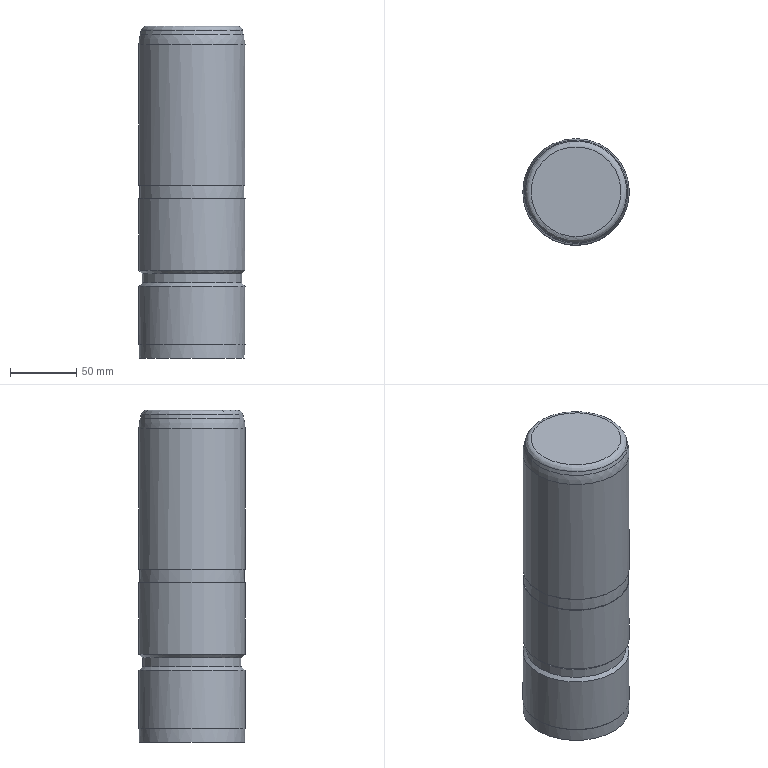Part | NX | features solid 2 | 1 solid | 16 faces | box 80 x 80 x 250 mm | volume 1244974 mm3 | cylinder 6 | plane 5 | cone 3 | torus 2 | commonest cylinder face diameters 80 x3 75 x1 79 x1 79.5 x1
STEP:
#1=CARTESIAN_POINT('',(1067.5,-565.,-201.5));
#2=VERTEX_POINT('',#1);
#3=CARTESIAN_POINT('',(1030.,-565.,-201.5));
#4=DIRECTION('',(0.,0.,-1.));
#5=DIRECTION('',(1.,0.,0.));
#6=AXIS2_PLACEMENT_3D('',#3,#4,#5);
#7=CIRCLE('',#6,37.5);
#8=EDGE_CURVE('',#2,#2,#7,.T.);
#9=ORIENTED_EDGE('',*,*,#8,.F.);
#10=EDGE_LOOP('',(#9));
#11=FACE_BOUND('',#10,.T.);
#12=CARTESIAN_POINT('',(990.,-565.,-199.));
#13=VERTEX_POINT('',#12);
#14=CARTESIAN_POINT('',(1030.,-565.,-199.));
#15=DIRECTION('',(0.,0.,1.));
#16=DIRECTION('',(-1.,0.,0.));
#17=AXIS2_PLACEMENT_3D('',#14,#15,#16);
#18=CIRCLE('',#17,40.);
#19=EDGE_CURVE('',#13,#13,#18,.T.);
#20=ORIENTED_EDGE('',*,*,#19,.F.);
#21=EDGE_LOOP('',(#20));
#22=FACE_BOUND('',#21,.T.);
#23=CARTESIAN_POINT('',(1030.,-565.,-201.5));
#24=DIRECTION('',(0.,0.,1.));
#25=DIRECTION('',(-1.,0.,0.));
#26=AXIS2_PLACEMENT_3D('',#23,#24,#25);
#27=CONICAL_SURFACE('',#26,37.5,0.7854);
#28=ADVANCED_FACE('',(#11,#22),#27,.T.);
#29=ORIENTED_EDGE('',*,*,#8,.T.);
#30=EDGE_LOOP('',(#29));
#31=FACE_BOUND('',#30,.T.);
#32=CARTESIAN_POINT('',(1067.5,-565.,-208.5));
#33=VERTEX_POINT('',#32);
#34=CARTESIAN_POINT('',(1030.,-565.,-208.5));
#35=DIRECTION('',(0.,0.,-1.));
#36=DIRECTION('',(1.,0.,0.));
#37=AXIS2_PLACEMENT_3D('',#34,#35,#36);
#38=CIRCLE('',#37,37.5);
#39=EDGE_CURVE('',#33,#33,#38,.T.);
#40=ORIENTED_EDGE('',*,*,#39,.F.);
#41=EDGE_LOOP('',(#40));
#42=FACE_BOUND('',#41,.T.);
#43=CARTESIAN_POINT('',(1030.,-565.,-208.5));
#44=DIRECTION('',(0.,0.,1.));
#45=DIRECTION('',(-1.,0.,0.));
#46=AXIS2_PLACEMENT_3D('',#43,#44,#45);
#47=CYLINDRICAL_SURFACE('',#46,37.5);
#48=ADVANCED_FACE('',(#31,#42),#47,.T.);
#49=CARTESIAN_POINT('',(990.5,-565.,-145.));
#50=VERTEX_POINT('',#49);
#51=CARTESIAN_POINT('',(1030.,-565.,-145.));
#52=DIRECTION('',(0.,0.,1.));
#53=DIRECTION('',(-1.,0.,0.));
#54=AXIS2_PLACEMENT_3D('',#51,#52,#53);
#55=CIRCLE('',#54,39.5);
#56=EDGE_CURVE('',#50,#50,#55,.T.);
#57=ORIENTED_EDGE('',*,*,#56,.F.);
#58=EDGE_LOOP('',(#57));
#59=FACE_BOUND('',#58,.T.);
#60=CARTESIAN_POINT('',(1070.,-565.,-145.));
#61=VERTEX_POINT('',#60);
#62=CARTESIAN_POINT('',(1030.,-565.,-145.));
#63=DIRECTION('',(0.,0.,-1.));
#64=DIRECTION('',(1.,0.,0.));
#65=AXIS2_PLACEMENT_3D('',#62,#63,#64);
#66=CIRCLE('',#65,40.);
#67=EDGE_CURVE('',#61,#61,#66,.T.);
#68=ORIENTED_EDGE('',*,*,#67,.F.);
#69=EDGE_LOOP('',(#68));
#70=FACE_BOUND('',#69,.T.);
#71=CARTESIAN_POINT('',(1030.,-565.,-145.));
#72=DIRECTION('',(0.,0.,1.));
#73=DIRECTION('',(-1.,0.,0.));
#74=AXIS2_PLACEMENT_3D('',#71,#72,#73);
#75=PLANE('',#74);
#76=ADVANCED_FACE('',(#59,#70),#75,.T.);
#77=ORIENTED_EDGE('',*,*,#67,.T.);
#78=EDGE_LOOP('',(#77));
#79=FACE_BOUND('',#78,.T.);
#80=ORIENTED_EDGE('',*,*,#19,.T.);
#81=EDGE_LOOP('',(#80));
#82=FACE_BOUND('',#81,.T.);
#83=CARTESIAN_POINT('',(1030.,-565.,-199.));
#84=DIRECTION('',(0.,0.,1.));
#85=DIRECTION('',(-1.,0.,0.));
#86=AXIS2_PLACEMENT_3D('',#83,#84,#85);
#87=CYLINDRICAL_SURFACE('',#86,40.);
#88=ADVANCED_FACE('',(#79,#82),#87,.T.);
#89=CARTESIAN_POINT('',(1069.5,-565.,-135.));
#90=VERTEX_POINT('',#89);
#91=CARTESIAN_POINT('',(1030.,-565.,-135.));
#92=DIRECTION('',(0.,0.,-1.));
#93=DIRECTION('',(1.,0.,0.));
#94=AXIS2_PLACEMENT_3D('',#91,#92,#93);
#95=CIRCLE('',#94,39.5);
#96=EDGE_CURVE('',#90,#90,#95,.T.);
#97=ORIENTED_EDGE('',*,*,#96,.F.);
#98=EDGE_LOOP('',(#97));
#99=FACE_BOUND('',#98,.T.);
#100=CARTESIAN_POINT('',(990.,-565.,-135.));
#101=VERTEX_POINT('',#100);
#102=CARTESIAN_POINT('',(1030.,-565.,-135.));
#103=DIRECTION('',(0.,0.,1.));
#104=DIRECTION('',(-1.,0.,0.));
#105=AXIS2_PLACEMENT_3D('',#102,#103,#104);
#106=CIRCLE('',#105,40.);
#107=EDGE_CURVE('',#101,#101,#106,.T.);
#108=ORIENTED_EDGE('',*,*,#107,.F.);
#109=EDGE_LOOP('',(#108));
#110=FACE_BOUND('',#109,.T.);
#111=CARTESIAN_POINT('',(1030.,-565.,-135.));
#112=DIRECTION('',(0.,0.,-1.));
#113=DIRECTION('',(1.,0.,0.));
#114=AXIS2_PLACEMENT_3D('',#111,#112,#113);
#115=PLANE('',#114);
#116=ADVANCED_FACE('',(#99,#110),#115,.T.);
#117=CARTESIAN_POINT('',(1070.,-565.,-28.95));
#118=VERTEX_POINT('',#117);
#119=CARTESIAN_POINT('',(1030.,-565.,-28.95));
#120=DIRECTION('',(0.,0.,-1.));
#121=DIRECTION('',(1.,0.,0.));
#122=AXIS2_PLACEMENT_3D('',#119,#120,#121);
#123=CIRCLE('',#122,40.);
#124=EDGE_CURVE('',#118,#118,#123,.T.);
#125=ORIENTED_EDGE('',*,*,#124,.T.);
#126=EDGE_LOOP('',(#125));
#127=FACE_BOUND('',#126,.T.);
#128=ORIENTED_EDGE('',*,*,#107,.T.);
#129=EDGE_LOOP('',(#128));
#130=FACE_BOUND('',#129,.T.);
#131=CARTESIAN_POINT('',(1030.,-565.,-135.));
#132=DIRECTION('',(0.,0.,1.));
#133=DIRECTION('',(-1.,0.,0.));
#134=AXIS2_PLACEMENT_3D('',#131,#132,#133);
#135=CYLINDRICAL_SURFACE('',#134,40.);
#136=ADVANCED_FACE('',(#127,#130),#135,.T.);
#137=ORIENTED_EDGE('',*,*,#96,.T.);
#138=EDGE_LOOP('',(#137));
#139=FACE_BOUND('',#138,.T.);
#140=ORIENTED_EDGE('',*,*,#56,.T.);
#141=EDGE_LOOP('',(#140));
#142=FACE_BOUND('',#141,.T.);
#143=CARTESIAN_POINT('',(1030.,-565.,-145.));
#144=DIRECTION('',(0.,0.,1.));
#145=DIRECTION('',(-1.,0.,0.));
#146=AXIS2_PLACEMENT_3D('',#143,#144,#145);
#147=CYLINDRICAL_SURFACE('',#146,39.5);
#148=ADVANCED_FACE('',(#139,#142),#147,.T.);
#149=CARTESIAN_POINT('',(996.132,-565.,-15.));
#150=VERTEX_POINT('',#149);
#151=CARTESIAN_POINT('',(1030.,-565.,-15.));
#152=DIRECTION('',(0.,0.,1.));
#153=DIRECTION('',(-1.,0.,0.));
#154=AXIS2_PLACEMENT_3D('',#151,#152,#153);
#155=CIRCLE('',#154,33.868);
#156=EDGE_CURVE('',#150,#150,#155,.T.);
#157=ORIENTED_EDGE('',*,*,#156,.T.);
#158=EDGE_LOOP('',(#157));
#159=FACE_BOUND('',#158,.T.);
#160=CARTESIAN_POINT('',(1030.,-565.,-15.));
#161=DIRECTION('',(0.,0.,1.));
#162=DIRECTION('',(-1.,0.,0.));
#163=AXIS2_PLACEMENT_3D('',#160,#161,#162);
#164=PLANE('',#163);
#165=ADVANCED_FACE('',(#159),#164,.T.);
#166=CARTESIAN_POINT('',(991.786,-565.,-18.335));
#167=VERTEX_POINT('',#166);
#168=CARTESIAN_POINT('',(1030.,-565.,-18.335));
#169=DIRECTION('',(0.,0.,1.));
#170=DIRECTION('',(-1.,0.,0.));
#171=AXIS2_PLACEMENT_3D('',#168,#169,#170);
#172=CIRCLE('',#171,38.214);
#173=EDGE_CURVE('',#167,#167,#172,.F.);
#174=ORIENTED_EDGE('',*,*,#173,.T.);
#175=EDGE_LOOP('',(#174));
#176=FACE_BOUND('',#175,.T.);
#177=CARTESIAN_POINT('',(991.022,-565.,-21.185));
#178=VERTEX_POINT('',#177);
#179=CARTESIAN_POINT('',(1030.,-565.,-21.185));
#180=DIRECTION('',(0.,0.,1.));
#181=DIRECTION('',(-1.,0.,0.));
#182=AXIS2_PLACEMENT_3D('',#179,#180,#181);
#183=CIRCLE('',#182,38.978);
#184=EDGE_CURVE('',#178,#178,#183,.T.);
#185=ORIENTED_EDGE('',*,*,#184,.T.);
#186=EDGE_LOOP('',(#185));
#187=FACE_BOUND('',#186,.T.);
#188=CARTESIAN_POINT('',(1030.,-565.,-15.));
#189=DIRECTION('',(0.,0.,-1.));
#190=DIRECTION('',(1.,0.,0.));
#191=AXIS2_PLACEMENT_3D('',#188,#189,#190);
#192=CONICAL_SURFACE('',#191,37.321,0.2618);
#193=ADVANCED_FACE('',(#176,#187),#192,.T.);
#194=CARTESIAN_POINT('',(1069.75,-565.,-255.));
#195=VERTEX_POINT('',#194);
#196=CARTESIAN_POINT('',(1030.,-565.,-255.));
#197=DIRECTION('',(0.,0.,-1.));
#198=DIRECTION('',(1.,0.,0.));
#199=AXIS2_PLACEMENT_3D('',#196,#197,#198);
#200=CIRCLE('',#199,39.75);
#201=EDGE_CURVE('',#195,#195,#200,.T.);
#202=ORIENTED_EDGE('',*,*,#201,.F.);
#203=EDGE_LOOP('',(#202));
#204=FACE_BOUND('',#203,.T.);
#205=CARTESIAN_POINT('',(990.,-565.,-255.));
#206=VERTEX_POINT('',#205);
#207=CARTESIAN_POINT('',(1030.,-565.,-255.));
#208=DIRECTION('',(0.,0.,1.));
#209=DIRECTION('',(-1.,0.,0.));
#210=AXIS2_PLACEMENT_3D('',#207,#208,#209);
#211=CIRCLE('',#210,40.);
#212=EDGE_CURVE('',#206,#206,#211,.T.);
#213=ORIENTED_EDGE('',*,*,#212,.F.);
#214=EDGE_LOOP('',(#213));
#215=FACE_BOUND('',#214,.T.);
#216=CARTESIAN_POINT('',(1030.,-565.,-255.));
#217=DIRECTION('',(0.,0.,-1.));
#218=DIRECTION('',(1.,0.,0.));
#219=AXIS2_PLACEMENT_3D('',#216,#217,#218);
#220=PLANE('',#219);
#221=ADVANCED_FACE('',(#204,#215),#220,.T.);
#222=CARTESIAN_POINT('',(990.,-565.,-211.));
#223=VERTEX_POINT('',#222);
#224=CARTESIAN_POINT('',(1030.,-565.,-211.));
#225=DIRECTION('',(0.,0.,1.));
#226=DIRECTION('',(-1.,0.,0.));
#227=AXIS2_PLACEMENT_3D('',#224,#225,#226);
#228=CIRCLE('',#227,40.);
#229=EDGE_CURVE('',#223,#223,#228,.T.);
#230=ORIENTED_EDGE('',*,*,#229,.F.);
#231=EDGE_LOOP('',(#230));
#232=FACE_BOUND('',#231,.T.);
#233=ORIENTED_EDGE('',*,*,#212,.T.);
#234=EDGE_LOOP('',(#233));
#235=FACE_BOUND('',#234,.T.);
#236=CARTESIAN_POINT('',(1030.,-565.,-255.));
#237=DIRECTION('',(0.,0.,1.));
#238=DIRECTION('',(-1.,0.,0.));
#239=AXIS2_PLACEMENT_3D('',#236,#237,#238);
#240=CYLINDRICAL_SURFACE('',#239,40.);
#241=ADVANCED_FACE('',(#232,#235),#240,.T.);
#242=CARTESIAN_POINT('',(990.25,-565.,-265.));
#243=VERTEX_POINT('',#242);
#244=CARTESIAN_POINT('',(1030.,-565.,-265.));
#245=DIRECTION('',(0.,0.,1.));
#246=DIRECTION('',(-1.,0.,0.));
#247=AXIS2_PLACEMENT_3D('',#244,#245,#246);
#248=CIRCLE('',#247,39.75);
#249=EDGE_CURVE('',#243,#243,#248,.T.);
#250=ORIENTED_EDGE('',*,*,#249,.F.);
#251=EDGE_LOOP('',(#250));
#252=FACE_BOUND('',#251,.T.);
#253=CARTESIAN_POINT('',(1030.,-565.,-265.));
#254=DIRECTION('',(0.,0.,-1.));
#255=DIRECTION('',(1.,0.,0.));
#256=AXIS2_PLACEMENT_3D('',#253,#254,#255);
#257=PLANE('',#256);
#258=ADVANCED_FACE('',(#252),#257,.T.);
#259=ORIENTED_EDGE('',*,*,#201,.T.);
#260=EDGE_LOOP('',(#259));
#261=FACE_BOUND('',#260,.T.);
#262=ORIENTED_EDGE('',*,*,#249,.T.);
#263=EDGE_LOOP('',(#262));
#264=FACE_BOUND('',#263,.T.);
#265=CARTESIAN_POINT('',(1030.,-565.,-265.));
#266=DIRECTION('',(0.,0.,1.));
#267=DIRECTION('',(-1.,0.,0.));
#268=AXIS2_PLACEMENT_3D('',#265,#266,#267);
#269=CYLINDRICAL_SURFACE('',#268,39.75);
#270=ADVANCED_FACE('',(#261,#264),#269,.T.);
#271=ORIENTED_EDGE('',*,*,#229,.T.);
#272=EDGE_LOOP('',(#271));
#273=FACE_BOUND('',#272,.T.);
#274=ORIENTED_EDGE('',*,*,#39,.T.);
#275=EDGE_LOOP('',(#274));
#276=FACE_BOUND('',#275,.T.);
#277=CARTESIAN_POINT('',(1030.,-565.,-208.5));
#278=DIRECTION('',(0.,0.,-1.));
#279=DIRECTION('',(1.,0.,0.));
#280=AXIS2_PLACEMENT_3D('',#277,#278,#279);
#281=CONICAL_SURFACE('',#280,37.5,0.7854);
#282=ADVANCED_FACE('',(#273,#276),#281,.T.);
#283=ORIENTED_EDGE('',*,*,#124,.F.);
#284=EDGE_LOOP('',(#283));
#285=FACE_BOUND('',#284,.T.);
#286=ORIENTED_EDGE('',*,*,#184,.F.);
#287=EDGE_LOOP('',(#286));
#288=FACE_BOUND('',#287,.T.);
#289=CARTESIAN_POINT('',(1030.,-565.,-28.95));
#290=DIRECTION('',(0.,0.,-1.));
#291=DIRECTION('',(1.,0.,0.));
#292=AXIS2_PLACEMENT_3D('',#289,#290,#291);
#293=DEGENERATE_TOROIDAL_SURFACE('',#292,10.,30.,.T.);
#294=ADVANCED_FACE('',(#285,#288),#293,.T.);
#295=ORIENTED_EDGE('',*,*,#156,.F.);
#296=EDGE_LOOP('',(#295));
#297=FACE_BOUND('',#296,.T.);
#298=ORIENTED_EDGE('',*,*,#173,.F.);
#299=EDGE_LOOP('',(#298));
#300=FACE_BOUND('',#299,.T.);
#301=CARTESIAN_POINT('',(1030.,-565.,-19.5));
#302=DIRECTION('',(0.,0.,1.));
#303=DIRECTION('',(-1.,0.,0.));
#304=AXIS2_PLACEMENT_3D('',#301,#302,#303);
#305=TOROIDAL_SURFACE('',#304,33.868,4.5);
#306=ADVANCED_FACE('',(#297,#300),#305,.T.);
#307=CLOSED_SHELL('',(#28,#48,#76,#88,#116,#136,#148,#165,#193,#221,#241,#258,#270,#282,#294,#306));
#308=MANIFOLD_SOLID_BREP('',#307);
#309=(LENGTH_UNIT()NAMED_UNIT(*)SI_UNIT(.MILLI.,.METRE.));
#310=UNCERTAINTY_MEASURE_WITH_UNIT(LENGTH_MEASURE(0.00001),#309,'','');
#311=(NAMED_UNIT(*)PLANE_ANGLE_UNIT()SI_UNIT($,.RADIAN.));
#312=(NAMED_UNIT(*)SI_UNIT($,.STERADIAN.)SOLID_ANGLE_UNIT());
#313=(GEOMETRIC_REPRESENTATION_CONTEXT(3)GLOBAL_UNCERTAINTY_ASSIGNED_CONTEXT((#310))GLOBAL_UNIT_ASSIGNED_CONTEXT((#309,#311,#312))REPRESENTATION_CONTEXT('',''));
#314=ADVANCED_BREP_SHAPE_REPRESENTATION('',(#308),#313);